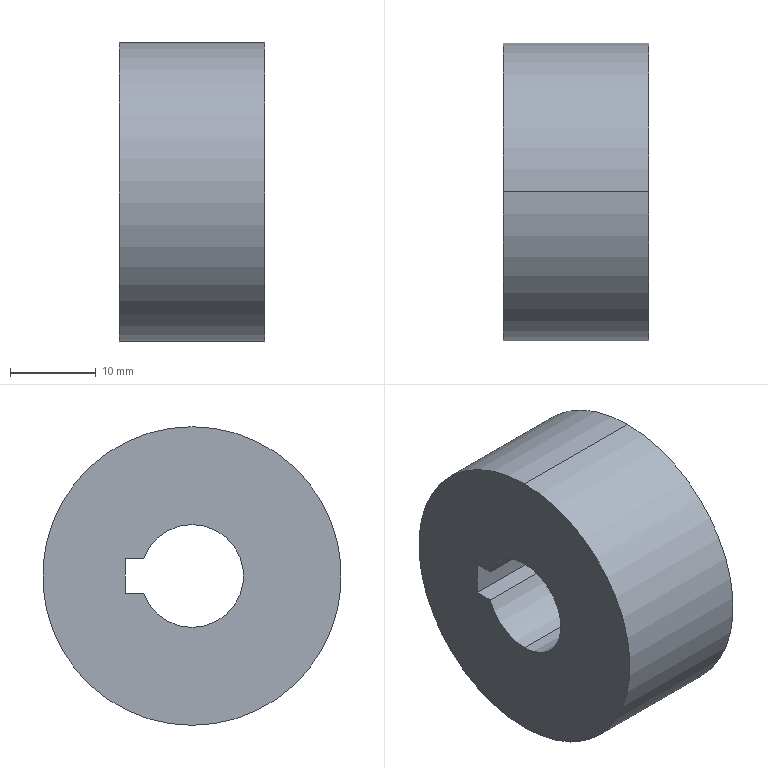Part | SolidWorks | features BaseBody 1, ICE 1 | 1 solid | 10 faces | box 17 x 34.83 x 34.83 mm | volume 14145 mm3 | cylinder 5 | plane 5 | commonest cylinder face diameters 12 x3 34.83 x2
STEP:
#1=CARTESIAN_POINT('',(-17.,5.657,-2.));
#2=VERTEX_POINT('',#1);
#3=CARTESIAN_POINT('',(-17.,0.,-6.));
#4=VERTEX_POINT('',#3);
#5=CARTESIAN_POINT('',(-17.,0.,0.));
#6=DIRECTION('',(-1.,0.,0.));
#7=DIRECTION('',(0.,0.,-1.));
#8=AXIS2_PLACEMENT_3D('',#5,#6,#7);
#9=CIRCLE('',#8,6.);
#10=EDGE_CURVE('',#2,#4,#9,.T.);
#11=ORIENTED_EDGE('',*,*,#10,.T.);
#12=CARTESIAN_POINT('',(0.,0.,-6.));
#13=VERTEX_POINT('',#12);
#14=CARTESIAN_POINT('',(29.,0.,-6.));
#15=DIRECTION('',(1.,0.,0.));
#16=VECTOR('',#15,1000.);
#17=LINE('',#14,#16);
#18=EDGE_CURVE('',#4,#13,#17,.T.);
#19=ORIENTED_EDGE('',*,*,#18,.T.);
#20=CARTESIAN_POINT('',(0.,5.657,-2.));
#21=VERTEX_POINT('',#20);
#22=CARTESIAN_POINT('',(0.,0.,0.));
#23=DIRECTION('',(1.,0.,0.));
#24=DIRECTION('',(0.,0.,1.));
#25=AXIS2_PLACEMENT_3D('',#22,#23,#24);
#26=CIRCLE('',#25,6.);
#27=EDGE_CURVE('',#13,#21,#26,.T.);
#28=ORIENTED_EDGE('',*,*,#27,.T.);
#29=CARTESIAN_POINT('',(29.,5.657,-2.));
#30=DIRECTION('',(-1.,0.,0.));
#31=VECTOR('',#30,1000.);
#32=LINE('',#29,#31);
#33=EDGE_CURVE('',#21,#2,#32,.T.);
#34=ORIENTED_EDGE('',*,*,#33,.T.);
#35=EDGE_LOOP('',(#11,#19,#28,#34));
#36=FACE_OUTER_BOUND('',#35,.T.);
#37=CARTESIAN_POINT('',(29.,0.,0.));
#38=DIRECTION('',(1.,0.,0.));
#39=DIRECTION('',(0.,0.,1.));
#40=AXIS2_PLACEMENT_3D('',#37,#38,#39);
#41=CYLINDRICAL_SURFACE('',#40,6.);
#42=ADVANCED_FACE('',(#36),#41,.F.);
#43=ORIENTED_EDGE('',*,*,#18,.F.);
#44=CARTESIAN_POINT('',(-17.,0.,6.));
#45=VERTEX_POINT('',#44);
#46=CARTESIAN_POINT('',(-17.,0.,0.));
#47=DIRECTION('',(-1.,0.,0.));
#48=DIRECTION('',(0.,0.,-1.));
#49=AXIS2_PLACEMENT_3D('',#46,#47,#48);
#50=CIRCLE('',#49,6.);
#51=EDGE_CURVE('',#4,#45,#50,.T.);
#52=ORIENTED_EDGE('',*,*,#51,.T.);
#53=CARTESIAN_POINT('',(0.,0.,6.));
#54=VERTEX_POINT('',#53);
#55=CARTESIAN_POINT('',(29.,0.,6.));
#56=DIRECTION('',(1.,0.,0.));
#57=VECTOR('',#56,1000.);
#58=LINE('',#55,#57);
#59=EDGE_CURVE('',#45,#54,#58,.T.);
#60=ORIENTED_EDGE('',*,*,#59,.T.);
#61=CARTESIAN_POINT('',(0.,0.,0.));
#62=DIRECTION('',(1.,0.,0.));
#63=DIRECTION('',(0.,0.,1.));
#64=AXIS2_PLACEMENT_3D('',#61,#62,#63);
#65=CIRCLE('',#64,6.);
#66=EDGE_CURVE('',#54,#13,#65,.T.);
#67=ORIENTED_EDGE('',*,*,#66,.T.);
#68=EDGE_LOOP('',(#43,#52,#60,#67));
#69=FACE_OUTER_BOUND('',#68,.T.);
#70=CARTESIAN_POINT('',(29.,0.,0.));
#71=DIRECTION('',(1.,0.,0.));
#72=DIRECTION('',(0.,0.,1.));
#73=AXIS2_PLACEMENT_3D('',#70,#71,#72);
#74=CYLINDRICAL_SURFACE('',#73,6.);
#75=ADVANCED_FACE('',(#69),#74,.F.);
#76=CARTESIAN_POINT('',(0.,0.,17.415));
#77=VERTEX_POINT('',#76);
#78=CARTESIAN_POINT('',(0.,0.,-17.415));
#79=VERTEX_POINT('',#78);
#80=CARTESIAN_POINT('',(0.,0.,0.));
#81=DIRECTION('',(1.,0.,0.));
#82=DIRECTION('',(0.,0.,-1.));
#83=AXIS2_PLACEMENT_3D('',#80,#81,#82);
#84=CIRCLE('',#83,17.415);
#85=EDGE_CURVE('',#77,#79,#84,.T.);
#86=ORIENTED_EDGE('',*,*,#85,.F.);
#87=CARTESIAN_POINT('',(-17.,0.,17.415));
#88=VERTEX_POINT('',#87);
#89=CARTESIAN_POINT('',(12.,0.,17.415));
#90=DIRECTION('',(-1.,0.,0.));
#91=VECTOR('',#90,1000.);
#92=LINE('',#89,#91);
#93=EDGE_CURVE('',#77,#88,#92,.T.);
#94=ORIENTED_EDGE('',*,*,#93,.T.);
#95=CARTESIAN_POINT('',(-17.,0.,-17.415));
#96=VERTEX_POINT('',#95);
#97=CARTESIAN_POINT('',(-17.,0.,0.));
#98=DIRECTION('',(1.,0.,0.));
#99=DIRECTION('',(0.,0.,-1.));
#100=AXIS2_PLACEMENT_3D('',#97,#98,#99);
#101=CIRCLE('',#100,17.415);
#102=EDGE_CURVE('',#88,#96,#101,.T.);
#103=ORIENTED_EDGE('',*,*,#102,.T.);
#104=CARTESIAN_POINT('',(12.,0.,-17.415));
#105=DIRECTION('',(-1.,0.,0.));
#106=VECTOR('',#105,1000.);
#107=LINE('',#104,#106);
#108=EDGE_CURVE('',#79,#96,#107,.T.);
#109=ORIENTED_EDGE('',*,*,#108,.F.);
#110=EDGE_LOOP('',(#86,#94,#103,#109));
#111=FACE_OUTER_BOUND('',#110,.T.);
#112=CARTESIAN_POINT('',(12.,0.,0.));
#113=DIRECTION('',(-1.,0.,0.));
#114=DIRECTION('',(0.,0.,-1.));
#115=AXIS2_PLACEMENT_3D('',#112,#113,#114);
#116=CYLINDRICAL_SURFACE('',#115,17.415);
#117=ADVANCED_FACE('',(#111),#116,.T.);
#118=CARTESIAN_POINT('',(0.,0.,0.));
#119=DIRECTION('',(1.,0.,0.));
#120=DIRECTION('',(0.,0.,-1.));
#121=AXIS2_PLACEMENT_3D('',#118,#119,#120);
#122=CIRCLE('',#121,17.415);
#123=EDGE_CURVE('',#79,#77,#122,.T.);
#124=ORIENTED_EDGE('',*,*,#123,.T.);
#125=ORIENTED_EDGE('',*,*,#85,.T.);
#126=EDGE_LOOP('',(#124,#125));
#127=FACE_OUTER_BOUND('',#126,.T.);
#128=CARTESIAN_POINT('',(0.,5.657,2.));
#129=VERTEX_POINT('',#128);
#130=CARTESIAN_POINT('',(0.,7.8,2.));
#131=VERTEX_POINT('',#130);
#132=CARTESIAN_POINT('',(0.,7.8,2.));
#133=DIRECTION('',(0.,1.,0.));
#134=VECTOR('',#133,1000.);
#135=LINE('',#132,#134);
#136=EDGE_CURVE('',#129,#131,#135,.T.);
#137=ORIENTED_EDGE('',*,*,#136,.T.);
#138=CARTESIAN_POINT('',(0.,7.8,-2.));
#139=VERTEX_POINT('',#138);
#140=CARTESIAN_POINT('',(0.,7.8,-2.));
#141=DIRECTION('',(0.,0.,-1.));
#142=VECTOR('',#141,1000.);
#143=LINE('',#140,#142);
#144=EDGE_CURVE('',#131,#139,#143,.T.);
#145=ORIENTED_EDGE('',*,*,#144,.T.);
#146=CARTESIAN_POINT('',(0.,5.657,-2.));
#147=DIRECTION('',(0.,-1.,0.));
#148=VECTOR('',#147,1000.);
#149=LINE('',#146,#148);
#150=EDGE_CURVE('',#139,#21,#149,.T.);
#151=ORIENTED_EDGE('',*,*,#150,.T.);
#152=ORIENTED_EDGE('',*,*,#27,.F.);
#153=ORIENTED_EDGE('',*,*,#66,.F.);
#154=CARTESIAN_POINT('',(0.,0.,0.));
#155=DIRECTION('',(1.,0.,0.));
#156=DIRECTION('',(0.,0.,1.));
#157=AXIS2_PLACEMENT_3D('',#154,#155,#156);
#158=CIRCLE('',#157,6.);
#159=EDGE_CURVE('',#129,#54,#158,.T.);
#160=ORIENTED_EDGE('',*,*,#159,.F.);
#161=EDGE_LOOP('',(#137,#145,#151,#152,#153,#160));
#162=FACE_BOUND('',#161,.T.);
#163=CARTESIAN_POINT('',(0.,0.,-17.415));
#164=DIRECTION('',(-1.,0.,0.));
#165=DIRECTION('',(0.,0.,1.));
#166=AXIS2_PLACEMENT_3D('',#163,#164,#165);
#167=PLANE('',#166);
#168=ADVANCED_FACE('',(#127,#162),#167,.F.);
#169=CARTESIAN_POINT('',(-17.,5.657,2.));
#170=VERTEX_POINT('',#169);
#171=CARTESIAN_POINT('',(-17.,7.8,2.));
#172=VERTEX_POINT('',#171);
#173=CARTESIAN_POINT('',(-17.,0.,2.));
#174=DIRECTION('',(0.,1.,0.));
#175=VECTOR('',#174,1000.);
#176=LINE('',#173,#175);
#177=EDGE_CURVE('',#170,#172,#176,.T.);
#178=ORIENTED_EDGE('',*,*,#177,.F.);
#179=CARTESIAN_POINT('',(-17.,0.,0.));
#180=DIRECTION('',(-1.,0.,0.));
#181=DIRECTION('',(0.,0.,-1.));
#182=AXIS2_PLACEMENT_3D('',#179,#180,#181);
#183=CIRCLE('',#182,6.);
#184=EDGE_CURVE('',#45,#170,#183,.T.);
#185=ORIENTED_EDGE('',*,*,#184,.F.);
#186=ORIENTED_EDGE('',*,*,#51,.F.);
#187=ORIENTED_EDGE('',*,*,#10,.F.);
#188=CARTESIAN_POINT('',(-17.,7.8,-2.));
#189=VERTEX_POINT('',#188);
#190=CARTESIAN_POINT('',(-17.,0.,-2.));
#191=DIRECTION('',(0.,-1.,0.));
#192=VECTOR('',#191,1000.);
#193=LINE('',#190,#192);
#194=EDGE_CURVE('',#189,#2,#193,.T.);
#195=ORIENTED_EDGE('',*,*,#194,.F.);
#196=CARTESIAN_POINT('',(-17.,7.8,0.));
#197=DIRECTION('',(0.,0.,-1.));
#198=VECTOR('',#197,1000.);
#199=LINE('',#196,#198);
#200=EDGE_CURVE('',#172,#189,#199,.T.);
#201=ORIENTED_EDGE('',*,*,#200,.F.);
#202=EDGE_LOOP('',(#178,#185,#186,#187,#195,#201));
#203=FACE_BOUND('',#202,.T.);
#204=CARTESIAN_POINT('',(-17.,0.,0.));
#205=DIRECTION('',(1.,0.,0.));
#206=DIRECTION('',(0.,0.,-1.));
#207=AXIS2_PLACEMENT_3D('',#204,#205,#206);
#208=CIRCLE('',#207,17.415);
#209=EDGE_CURVE('',#96,#88,#208,.T.);
#210=ORIENTED_EDGE('',*,*,#209,.F.);
#211=ORIENTED_EDGE('',*,*,#102,.F.);
#212=EDGE_LOOP('',(#210,#211));
#213=FACE_OUTER_BOUND('',#212,.T.);
#214=CARTESIAN_POINT('',(-17.,0.,0.));
#215=DIRECTION('',(1.,0.,0.));
#216=DIRECTION('',(0.,1.,0.));
#217=AXIS2_PLACEMENT_3D('',#214,#215,#216);
#218=PLANE('',#217);
#219=ADVANCED_FACE('',(#203,#213),#218,.F.);
#220=ORIENTED_EDGE('',*,*,#93,.F.);
#221=ORIENTED_EDGE('',*,*,#123,.F.);
#222=ORIENTED_EDGE('',*,*,#108,.T.);
#223=ORIENTED_EDGE('',*,*,#209,.T.);
#224=EDGE_LOOP('',(#220,#221,#222,#223));
#225=FACE_OUTER_BOUND('',#224,.T.);
#226=CARTESIAN_POINT('',(12.,0.,0.));
#227=DIRECTION('',(-1.,0.,0.));
#228=DIRECTION('',(0.,0.,-1.));
#229=AXIS2_PLACEMENT_3D('',#226,#227,#228);
#230=CYLINDRICAL_SURFACE('',#229,17.415);
#231=ADVANCED_FACE('',(#225),#230,.T.);
#232=ORIENTED_EDGE('',*,*,#136,.F.);
#233=CARTESIAN_POINT('',(29.,5.657,2.));
#234=DIRECTION('',(-1.,0.,0.));
#235=VECTOR('',#234,1000.);
#236=LINE('',#233,#235);
#237=EDGE_CURVE('',#129,#170,#236,.T.);
#238=ORIENTED_EDGE('',*,*,#237,.T.);
#239=ORIENTED_EDGE('',*,*,#177,.T.);
#240=CARTESIAN_POINT('',(29.,7.8,2.));
#241=DIRECTION('',(-1.,0.,0.));
#242=VECTOR('',#241,1000.);
#243=LINE('',#240,#242);
#244=EDGE_CURVE('',#131,#172,#243,.T.);
#245=ORIENTED_EDGE('',*,*,#244,.F.);
#246=EDGE_LOOP('',(#232,#238,#239,#245));
#247=FACE_OUTER_BOUND('',#246,.T.);
#248=CARTESIAN_POINT('',(29.,7.8,2.));
#249=DIRECTION('',(0.,0.,-1.));
#250=DIRECTION('',(0.,-1.,0.));
#251=AXIS2_PLACEMENT_3D('',#248,#249,#250);
#252=PLANE('',#251);
#253=ADVANCED_FACE('',(#247),#252,.T.);
#254=ORIENTED_EDGE('',*,*,#59,.F.);
#255=ORIENTED_EDGE('',*,*,#184,.T.);
#256=ORIENTED_EDGE('',*,*,#237,.F.);
#257=ORIENTED_EDGE('',*,*,#159,.T.);
#258=EDGE_LOOP('',(#254,#255,#256,#257));
#259=FACE_OUTER_BOUND('',#258,.T.);
#260=CARTESIAN_POINT('',(29.,0.,0.));
#261=DIRECTION('',(1.,0.,0.));
#262=DIRECTION('',(0.,0.,1.));
#263=AXIS2_PLACEMENT_3D('',#260,#261,#262);
#264=CYLINDRICAL_SURFACE('',#263,6.);
#265=ADVANCED_FACE('',(#259),#264,.F.);
#266=ORIENTED_EDGE('',*,*,#150,.F.);
#267=CARTESIAN_POINT('',(29.,7.8,-2.));
#268=DIRECTION('',(-1.,0.,0.));
#269=VECTOR('',#268,1000.);
#270=LINE('',#267,#269);
#271=EDGE_CURVE('',#139,#189,#270,.T.);
#272=ORIENTED_EDGE('',*,*,#271,.T.);
#273=ORIENTED_EDGE('',*,*,#194,.T.);
#274=ORIENTED_EDGE('',*,*,#33,.F.);
#275=EDGE_LOOP('',(#266,#272,#273,#274));
#276=FACE_OUTER_BOUND('',#275,.T.);
#277=CARTESIAN_POINT('',(29.,5.657,-2.));
#278=DIRECTION('',(0.,0.,1.));
#279=DIRECTION('',(1.,0.,0.));
#280=AXIS2_PLACEMENT_3D('',#277,#278,#279);
#281=PLANE('',#280);
#282=ADVANCED_FACE('',(#276),#281,.T.);
#283=ORIENTED_EDGE('',*,*,#144,.F.);
#284=ORIENTED_EDGE('',*,*,#244,.T.);
#285=ORIENTED_EDGE('',*,*,#200,.T.);
#286=ORIENTED_EDGE('',*,*,#271,.F.);
#287=EDGE_LOOP('',(#283,#284,#285,#286));
#288=FACE_OUTER_BOUND('',#287,.T.);
#289=CARTESIAN_POINT('',(29.,7.8,-2.));
#290=DIRECTION('',(0.,-1.,0.));
#291=DIRECTION('',(0.,0.,-1.));
#292=AXIS2_PLACEMENT_3D('',#289,#290,#291);
#293=PLANE('',#292);
#294=ADVANCED_FACE('',(#288),#293,.T.);
#295=CLOSED_SHELL('',(#42,#75,#117,#168,#219,#231,#253,#265,#282,#294));
#296=MANIFOLD_SOLID_BREP('',#295);
#297=CARTESIAN_POINT('',(0.,0.,0.));
#298=DIRECTION('',(0.,0.,1.));
#299=DIRECTION('',(1.,0.,0.));
#300=AXIS2_PLACEMENT_3D('',#297,#298,#299);
#301=(LENGTH_UNIT()NAMED_UNIT(*)SI_UNIT(.MILLI.,.METRE.));
#302=UNCERTAINTY_MEASURE_WITH_UNIT(LENGTH_MEASURE(0.00001),#301,'','');
#303=(NAMED_UNIT(*)PLANE_ANGLE_UNIT()SI_UNIT($,.RADIAN.));
#304=(NAMED_UNIT(*)SI_UNIT($,.STERADIAN.)SOLID_ANGLE_UNIT());
#305=(GEOMETRIC_REPRESENTATION_CONTEXT(3)GLOBAL_UNCERTAINTY_ASSIGNED_CONTEXT((#302))GLOBAL_UNIT_ASSIGNED_CONTEXT((#301,#303,#304))REPRESENTATION_CONTEXT('',''));
#306=ADVANCED_BREP_SHAPE_REPRESENTATION('',(#296,#300),#305);